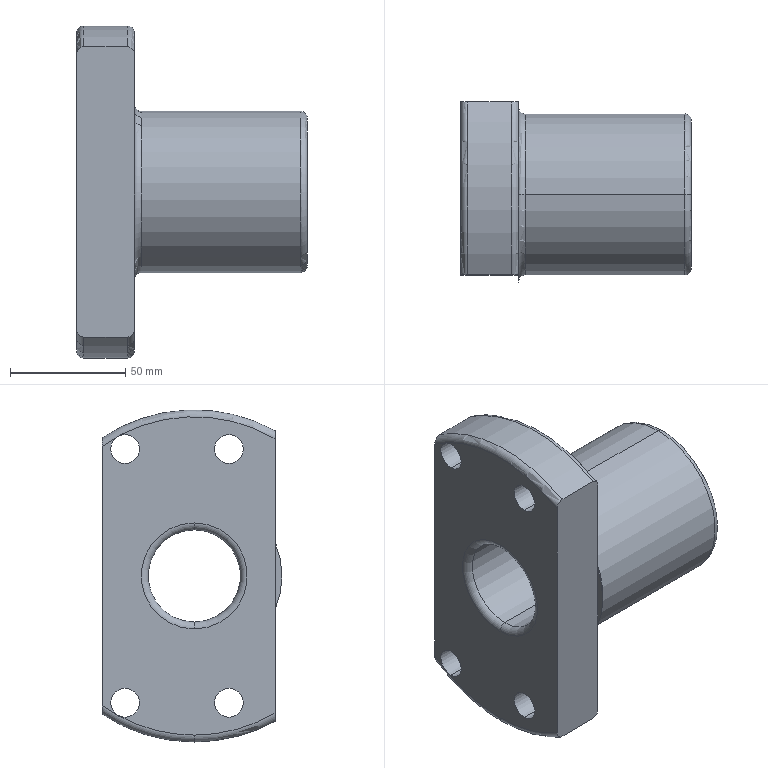Part | SolidWorks | features BaseBody 1 | 1 solid | 35 faces | box 100 x 78 x 144 mm | volume 406652 mm3 | cylinder 15 | torus 14 | plane 6 | commonest cylinder face diameters 12.5 x8 144 x3 40 x2 70 x2
STEP:
#1=CARTESIAN_POINT('',(-75.,30.,-48.75));
#2=VERTEX_POINT('',#1);
#3=CARTESIAN_POINT('',(-75.,30.,-61.25));
#4=VERTEX_POINT('',#3);
#5=CARTESIAN_POINT('',(-75.,30.,-55.));
#6=DIRECTION('',(1.,0.,0.));
#7=DIRECTION('',(0.,0.,-1.));
#8=AXIS2_PLACEMENT_3D('',#5,#6,#7);
#9=CIRCLE('',#8,6.25);
#10=EDGE_CURVE('',#2,#4,#9,.T.);
#11=ORIENTED_EDGE('',*,*,#10,.T.);
#12=CARTESIAN_POINT('',(-100.,30.,-61.25));
#13=VERTEX_POINT('',#12);
#14=CARTESIAN_POINT('',(-70.,30.,-61.25));
#15=DIRECTION('',(-1.,0.,0.));
#16=VECTOR('',#15,1000.);
#17=LINE('',#14,#16);
#18=EDGE_CURVE('',#4,#13,#17,.T.);
#19=ORIENTED_EDGE('',*,*,#18,.T.);
#20=CARTESIAN_POINT('',(-100.,30.,-48.75));
#21=VERTEX_POINT('',#20);
#22=CARTESIAN_POINT('',(-100.,30.,-55.));
#23=DIRECTION('',(-1.,0.,0.));
#24=DIRECTION('',(0.,0.,1.));
#25=AXIS2_PLACEMENT_3D('',#22,#23,#24);
#26=CIRCLE('',#25,6.25);
#27=EDGE_CURVE('',#13,#21,#26,.T.);
#28=ORIENTED_EDGE('',*,*,#27,.T.);
#29=CARTESIAN_POINT('',(-70.,30.,-48.75));
#30=DIRECTION('',(-1.,0.,0.));
#31=VECTOR('',#30,1000.);
#32=LINE('',#29,#31);
#33=EDGE_CURVE('',#2,#21,#32,.T.);
#34=ORIENTED_EDGE('',*,*,#33,.F.);
#35=EDGE_LOOP('',(#11,#19,#28,#34));
#36=FACE_OUTER_BOUND('',#35,.T.);
#37=CARTESIAN_POINT('',(-70.,30.,-55.));
#38=DIRECTION('',(-1.,0.,0.));
#39=DIRECTION('',(0.,0.,1.));
#40=AXIS2_PLACEMENT_3D('',#37,#38,#39);
#41=CYLINDRICAL_SURFACE('',#40,6.25);
#42=ADVANCED_FACE('',(#36),#41,.F.);
#43=CARTESIAN_POINT('',(-75.,30.,61.25));
#44=VERTEX_POINT('',#43);
#45=CARTESIAN_POINT('',(-75.,30.,48.75));
#46=VERTEX_POINT('',#45);
#47=CARTESIAN_POINT('',(-75.,30.,55.));
#48=DIRECTION('',(1.,0.,0.));
#49=DIRECTION('',(0.,0.,-1.));
#50=AXIS2_PLACEMENT_3D('',#47,#48,#49);
#51=CIRCLE('',#50,6.25);
#52=EDGE_CURVE('',#44,#46,#51,.T.);
#53=ORIENTED_EDGE('',*,*,#52,.T.);
#54=CARTESIAN_POINT('',(-100.,30.,48.75));
#55=VERTEX_POINT('',#54);
#56=CARTESIAN_POINT('',(-70.,30.,48.75));
#57=DIRECTION('',(-1.,0.,0.));
#58=VECTOR('',#57,1000.);
#59=LINE('',#56,#58);
#60=EDGE_CURVE('',#46,#55,#59,.T.);
#61=ORIENTED_EDGE('',*,*,#60,.T.);
#62=CARTESIAN_POINT('',(-100.,30.,61.25));
#63=VERTEX_POINT('',#62);
#64=CARTESIAN_POINT('',(-100.,30.,55.));
#65=DIRECTION('',(-1.,0.,0.));
#66=DIRECTION('',(0.,0.,1.));
#67=AXIS2_PLACEMENT_3D('',#64,#65,#66);
#68=CIRCLE('',#67,6.25);
#69=EDGE_CURVE('',#55,#63,#68,.T.);
#70=ORIENTED_EDGE('',*,*,#69,.T.);
#71=CARTESIAN_POINT('',(-70.,30.,61.25));
#72=DIRECTION('',(-1.,0.,0.));
#73=VECTOR('',#72,1000.);
#74=LINE('',#71,#73);
#75=EDGE_CURVE('',#44,#63,#74,.T.);
#76=ORIENTED_EDGE('',*,*,#75,.F.);
#77=EDGE_LOOP('',(#53,#61,#70,#76));
#78=FACE_OUTER_BOUND('',#77,.T.);
#79=CARTESIAN_POINT('',(-70.,30.,55.));
#80=DIRECTION('',(-1.,0.,0.));
#81=DIRECTION('',(0.,0.,1.));
#82=AXIS2_PLACEMENT_3D('',#79,#80,#81);
#83=CYLINDRICAL_SURFACE('',#82,6.25);
#84=ADVANCED_FACE('',(#78),#83,.F.);
#85=CARTESIAN_POINT('',(-75.,-15.,61.25));
#86=VERTEX_POINT('',#85);
#87=CARTESIAN_POINT('',(-75.,-15.,48.75));
#88=VERTEX_POINT('',#87);
#89=CARTESIAN_POINT('',(-75.,-15.,55.));
#90=DIRECTION('',(1.,0.,0.));
#91=DIRECTION('',(0.,0.,-1.));
#92=AXIS2_PLACEMENT_3D('',#89,#90,#91);
#93=CIRCLE('',#92,6.25);
#94=EDGE_CURVE('',#86,#88,#93,.T.);
#95=ORIENTED_EDGE('',*,*,#94,.T.);
#96=CARTESIAN_POINT('',(-100.,-15.,48.75));
#97=VERTEX_POINT('',#96);
#98=CARTESIAN_POINT('',(-70.,-15.,48.75));
#99=DIRECTION('',(-1.,0.,0.));
#100=VECTOR('',#99,1000.);
#101=LINE('',#98,#100);
#102=EDGE_CURVE('',#88,#97,#101,.T.);
#103=ORIENTED_EDGE('',*,*,#102,.T.);
#104=CARTESIAN_POINT('',(-100.,-15.,61.25));
#105=VERTEX_POINT('',#104);
#106=CARTESIAN_POINT('',(-100.,-15.,55.));
#107=DIRECTION('',(-1.,0.,0.));
#108=DIRECTION('',(0.,0.,1.));
#109=AXIS2_PLACEMENT_3D('',#106,#107,#108);
#110=CIRCLE('',#109,6.25);
#111=EDGE_CURVE('',#97,#105,#110,.T.);
#112=ORIENTED_EDGE('',*,*,#111,.T.);
#113=CARTESIAN_POINT('',(-70.,-15.,61.25));
#114=DIRECTION('',(-1.,0.,0.));
#115=VECTOR('',#114,1000.);
#116=LINE('',#113,#115);
#117=EDGE_CURVE('',#86,#105,#116,.T.);
#118=ORIENTED_EDGE('',*,*,#117,.F.);
#119=EDGE_LOOP('',(#95,#103,#112,#118));
#120=FACE_OUTER_BOUND('',#119,.T.);
#121=CARTESIAN_POINT('',(-70.,-15.,55.));
#122=DIRECTION('',(-1.,0.,0.));
#123=DIRECTION('',(0.,0.,1.));
#124=AXIS2_PLACEMENT_3D('',#121,#122,#123);
#125=CYLINDRICAL_SURFACE('',#124,6.25);
#126=ADVANCED_FACE('',(#120),#125,.F.);
#127=CARTESIAN_POINT('',(-75.,-15.,-48.75));
#128=VERTEX_POINT('',#127);
#129=CARTESIAN_POINT('',(-75.,-15.,-61.25));
#130=VERTEX_POINT('',#129);
#131=CARTESIAN_POINT('',(-75.,-15.,-55.));
#132=DIRECTION('',(1.,0.,0.));
#133=DIRECTION('',(0.,0.,-1.));
#134=AXIS2_PLACEMENT_3D('',#131,#132,#133);
#135=CIRCLE('',#134,6.25);
#136=EDGE_CURVE('',#128,#130,#135,.T.);
#137=ORIENTED_EDGE('',*,*,#136,.T.);
#138=CARTESIAN_POINT('',(-100.,-15.,-61.25));
#139=VERTEX_POINT('',#138);
#140=CARTESIAN_POINT('',(-70.,-15.,-61.25));
#141=DIRECTION('',(-1.,0.,0.));
#142=VECTOR('',#141,1000.);
#143=LINE('',#140,#142);
#144=EDGE_CURVE('',#130,#139,#143,.T.);
#145=ORIENTED_EDGE('',*,*,#144,.T.);
#146=CARTESIAN_POINT('',(-100.,-15.,-48.75));
#147=VERTEX_POINT('',#146);
#148=CARTESIAN_POINT('',(-100.,-15.,-55.));
#149=DIRECTION('',(-1.,0.,0.));
#150=DIRECTION('',(0.,0.,1.));
#151=AXIS2_PLACEMENT_3D('',#148,#149,#150);
#152=CIRCLE('',#151,6.25);
#153=EDGE_CURVE('',#139,#147,#152,.T.);
#154=ORIENTED_EDGE('',*,*,#153,.T.);
#155=CARTESIAN_POINT('',(-70.,-15.,-48.75));
#156=DIRECTION('',(-1.,0.,0.));
#157=VECTOR('',#156,1000.);
#158=LINE('',#155,#157);
#159=EDGE_CURVE('',#128,#147,#158,.T.);
#160=ORIENTED_EDGE('',*,*,#159,.F.);
#161=EDGE_LOOP('',(#137,#145,#154,#160));
#162=FACE_OUTER_BOUND('',#161,.T.);
#163=CARTESIAN_POINT('',(-70.,-15.,-55.));
#164=DIRECTION('',(-1.,0.,0.));
#165=DIRECTION('',(0.,0.,1.));
#166=AXIS2_PLACEMENT_3D('',#163,#164,#165);
#167=CYLINDRICAL_SURFACE('',#166,6.25);
#168=ADVANCED_FACE('',(#162),#167,.F.);
#169=CARTESIAN_POINT('',(-3.,0.,-35.));
#170=VERTEX_POINT('',#169);
#171=CARTESIAN_POINT('',(-3.,0.,35.));
#172=VERTEX_POINT('',#171);
#173=CARTESIAN_POINT('',(-3.,0.,0.));
#174=DIRECTION('',(1.,0.,0.));
#175=DIRECTION('',(0.,0.,-1.));
#176=AXIS2_PLACEMENT_3D('',#173,#174,#175);
#177=CIRCLE('',#176,35.);
#178=EDGE_CURVE('',#170,#172,#177,.T.);
#179=ORIENTED_EDGE('',*,*,#178,.T.);
#180=CARTESIAN_POINT('',(0.,0.,32.));
#181=VERTEX_POINT('',#180);
#182=CARTESIAN_POINT('',(-3.,0.,32.));
#183=DIRECTION('',(0.,1.,0.));
#184=DIRECTION('',(0.,0.,1.));
#185=AXIS2_PLACEMENT_3D('',#182,#183,#184);
#186=CIRCLE('',#185,3.);
#187=EDGE_CURVE('',#172,#181,#186,.T.);
#188=ORIENTED_EDGE('',*,*,#187,.T.);
#189=CARTESIAN_POINT('',(0.,0.,-32.));
#190=VERTEX_POINT('',#189);
#191=CARTESIAN_POINT('',(0.,0.,0.));
#192=DIRECTION('',(1.,0.,0.));
#193=DIRECTION('',(0.,0.,-1.));
#194=AXIS2_PLACEMENT_3D('',#191,#192,#193);
#195=CIRCLE('',#194,32.);
#196=EDGE_CURVE('',#190,#181,#195,.T.);
#197=ORIENTED_EDGE('',*,*,#196,.F.);
#198=CARTESIAN_POINT('',(-3.,0.,-32.));
#199=DIRECTION('',(0.,-1.,0.));
#200=DIRECTION('',(0.,0.,-1.));
#201=AXIS2_PLACEMENT_3D('',#198,#199,#200);
#202=CIRCLE('',#201,3.);
#203=EDGE_CURVE('',#170,#190,#202,.T.);
#204=ORIENTED_EDGE('',*,*,#203,.F.);
#205=EDGE_LOOP('',(#179,#188,#197,#204));
#206=FACE_OUTER_BOUND('',#205,.T.);
#207=CARTESIAN_POINT('',(-3.,0.,0.));
#208=DIRECTION('',(1.,0.,0.));
#209=DIRECTION('',(0.,0.,-1.));
#210=AXIS2_PLACEMENT_3D('',#207,#208,#209);
#211=TOROIDAL_SURFACE('',#210,32.,3.);
#212=ADVANCED_FACE('',(#206),#211,.T.);
#213=CARTESIAN_POINT('',(-72.,0.,-35.));
#214=VERTEX_POINT('',#213);
#215=CARTESIAN_POINT('',(-72.,0.,35.));
#216=VERTEX_POINT('',#215);
#217=CARTESIAN_POINT('',(-72.,0.,0.));
#218=DIRECTION('',(1.,0.,0.));
#219=DIRECTION('',(0.,0.,-1.));
#220=AXIS2_PLACEMENT_3D('',#217,#218,#219);
#221=CIRCLE('',#220,35.);
#222=EDGE_CURVE('',#214,#216,#221,.T.);
#223=ORIENTED_EDGE('',*,*,#222,.T.);
#224=CARTESIAN_POINT('',(0.,0.,35.));
#225=DIRECTION('',(1.,0.,0.));
#226=VECTOR('',#225,1000.);
#227=LINE('',#224,#226);
#228=EDGE_CURVE('',#216,#172,#227,.T.);
#229=ORIENTED_EDGE('',*,*,#228,.T.);
#230=ORIENTED_EDGE('',*,*,#178,.F.);
#231=CARTESIAN_POINT('',(0.,0.,-35.));
#232=DIRECTION('',(1.,0.,0.));
#233=VECTOR('',#232,1000.);
#234=LINE('',#231,#233);
#235=EDGE_CURVE('',#214,#170,#234,.T.);
#236=ORIENTED_EDGE('',*,*,#235,.F.);
#237=EDGE_LOOP('',(#223,#229,#230,#236));
#238=FACE_OUTER_BOUND('',#237,.T.);
#239=CARTESIAN_POINT('',(0.,0.,0.));
#240=DIRECTION('',(1.,0.,0.));
#241=DIRECTION('',(0.,0.,-1.));
#242=AXIS2_PLACEMENT_3D('',#239,#240,#241);
#243=CYLINDRICAL_SURFACE('',#242,35.);
#244=ADVANCED_FACE('',(#238),#243,.T.);
#245=CARTESIAN_POINT('',(-72.,0.,0.));
#246=DIRECTION('',(1.,0.,0.));
#247=DIRECTION('',(0.,0.,-1.));
#248=AXIS2_PLACEMENT_3D('',#245,#246,#247);
#249=CIRCLE('',#248,35.);
#250=EDGE_CURVE('',#216,#214,#249,.T.);
#251=ORIENTED_EDGE('',*,*,#250,.F.);
#252=CARTESIAN_POINT('',(-75.,0.,38.));
#253=VERTEX_POINT('',#252);
#254=CARTESIAN_POINT('',(-72.,0.,38.));
#255=DIRECTION('',(0.,1.,0.));
#256=DIRECTION('',(0.,0.,1.));
#257=AXIS2_PLACEMENT_3D('',#254,#255,#256);
#258=CIRCLE('',#257,3.);
#259=EDGE_CURVE('',#216,#253,#258,.T.);
#260=ORIENTED_EDGE('',*,*,#259,.T.);
#261=CARTESIAN_POINT('',(-75.,-35.,14.799));
#262=VERTEX_POINT('',#261);
#263=CARTESIAN_POINT('',(-75.,0.,0.));
#264=DIRECTION('',(1.,0.,0.));
#265=DIRECTION('',(0.,0.,-1.));
#266=AXIS2_PLACEMENT_3D('',#263,#264,#265);
#267=CIRCLE('',#266,38.);
#268=EDGE_CURVE('',#253,#262,#267,.T.);
#269=ORIENTED_EDGE('',*,*,#268,.T.);
#270=CARTESIAN_POINT('',(-75.,-35.,-14.799));
#271=VERTEX_POINT('',#270);
#272=CARTESIAN_POINT('',(-75.,0.,0.));
#273=DIRECTION('',(1.,0.,0.));
#274=DIRECTION('',(0.,0.,-1.));
#275=AXIS2_PLACEMENT_3D('',#272,#273,#274);
#276=CIRCLE('',#275,38.);
#277=EDGE_CURVE('',#262,#271,#276,.T.);
#278=ORIENTED_EDGE('',*,*,#277,.T.);
#279=CARTESIAN_POINT('',(-75.,0.,-38.));
#280=VERTEX_POINT('',#279);
#281=CARTESIAN_POINT('',(-75.,0.,0.));
#282=DIRECTION('',(1.,0.,0.));
#283=DIRECTION('',(0.,0.,-1.));
#284=AXIS2_PLACEMENT_3D('',#281,#282,#283);
#285=CIRCLE('',#284,38.);
#286=EDGE_CURVE('',#271,#280,#285,.T.);
#287=ORIENTED_EDGE('',*,*,#286,.T.);
#288=CARTESIAN_POINT('',(-72.,0.,-38.));
#289=DIRECTION('',(0.,-1.,0.));
#290=DIRECTION('',(0.,0.,-1.));
#291=AXIS2_PLACEMENT_3D('',#288,#289,#290);
#292=CIRCLE('',#291,3.);
#293=EDGE_CURVE('',#214,#280,#292,.T.);
#294=ORIENTED_EDGE('',*,*,#293,.F.);
#295=EDGE_LOOP('',(#251,#260,#269,#278,#287,#294));
#296=FACE_OUTER_BOUND('',#295,.T.);
#297=CARTESIAN_POINT('',(-72.,0.,0.));
#298=DIRECTION('',(1.,0.,0.));
#299=DIRECTION('',(0.,0.,-1.));
#300=AXIS2_PLACEMENT_3D('',#297,#298,#299);
#301=TOROIDAL_SURFACE('',#300,38.,3.);
#302=ADVANCED_FACE('',(#296),#301,.F.);
#303=CARTESIAN_POINT('',(-97.,0.,-20.));
#304=VERTEX_POINT('',#303);
#305=CARTESIAN_POINT('',(-97.,0.,20.));
#306=VERTEX_POINT('',#305);
#307=CARTESIAN_POINT('',(-97.,0.,0.));
#308=DIRECTION('',(1.,0.,0.));
#309=DIRECTION('',(0.,0.,-1.));
#310=AXIS2_PLACEMENT_3D('',#307,#308,#309);
#311=CIRCLE('',#310,20.);
#312=EDGE_CURVE('',#304,#306,#311,.T.);
#313=ORIENTED_EDGE('',*,*,#312,.T.);
#314=CARTESIAN_POINT('',(-100.,0.,23.));
#315=VERTEX_POINT('',#314);
#316=CARTESIAN_POINT('',(-97.,0.,23.));
#317=DIRECTION('',(0.,1.,0.));
#318=DIRECTION('',(0.,0.,1.));
#319=AXIS2_PLACEMENT_3D('',#316,#317,#318);
#320=CIRCLE('',#319,3.);
#321=EDGE_CURVE('',#306,#315,#320,.T.);
#322=ORIENTED_EDGE('',*,*,#321,.T.);
#323=CARTESIAN_POINT('',(-100.,0.,-23.));
#324=VERTEX_POINT('',#323);
#325=CARTESIAN_POINT('',(-100.,0.,0.));
#326=DIRECTION('',(1.,0.,0.));
#327=DIRECTION('',(0.,0.,-1.));
#328=AXIS2_PLACEMENT_3D('',#325,#326,#327);
#329=CIRCLE('',#328,23.);
#330=EDGE_CURVE('',#324,#315,#329,.T.);
#331=ORIENTED_EDGE('',*,*,#330,.F.);
#332=CARTESIAN_POINT('',(-97.,0.,-23.));
#333=DIRECTION('',(0.,-1.,0.));
#334=DIRECTION('',(0.,0.,-1.));
#335=AXIS2_PLACEMENT_3D('',#332,#333,#334);
#336=CIRCLE('',#335,3.);
#337=EDGE_CURVE('',#304,#324,#336,.T.);
#338=ORIENTED_EDGE('',*,*,#337,.F.);
#339=EDGE_LOOP('',(#313,#322,#331,#338));
#340=FACE_OUTER_BOUND('',#339,.T.);
#341=CARTESIAN_POINT('',(-97.,0.,0.));
#342=DIRECTION('',(1.,0.,0.));
#343=DIRECTION('',(0.,0.,-1.));
#344=AXIS2_PLACEMENT_3D('',#341,#342,#343);
#345=TOROIDAL_SURFACE('',#344,23.,3.);
#346=ADVANCED_FACE('',(#340),#345,.T.);
#347=CARTESIAN_POINT('',(-97.,0.,0.));
#348=DIRECTION('',(1.,0.,0.));
#349=DIRECTION('',(0.,0.,-1.));
#350=AXIS2_PLACEMENT_3D('',#347,#348,#349);
#351=CIRCLE('',#350,20.);
#352=EDGE_CURVE('',#306,#304,#351,.T.);
#353=ORIENTED_EDGE('',*,*,#352,.F.);
#354=CARTESIAN_POINT('',(-3.,0.,20.));
#355=VERTEX_POINT('',#354);
#356=CARTESIAN_POINT('',(0.,0.,20.));
#357=DIRECTION('',(1.,0.,0.));
#358=VECTOR('',#357,1000.);
#359=LINE('',#356,#358);
#360=EDGE_CURVE('',#306,#355,#359,.T.);
#361=ORIENTED_EDGE('',*,*,#360,.T.);
#362=CARTESIAN_POINT('',(-3.,0.,-20.));
#363=VERTEX_POINT('',#362);
#364=CARTESIAN_POINT('',(-3.,0.,0.));
#365=DIRECTION('',(1.,0.,0.));
#366=DIRECTION('',(0.,0.,-1.));
#367=AXIS2_PLACEMENT_3D('',#364,#365,#366);
#368=CIRCLE('',#367,20.);
#369=EDGE_CURVE('',#355,#363,#368,.T.);
#370=ORIENTED_EDGE('',*,*,#369,.T.);
#371=CARTESIAN_POINT('',(0.,0.,-20.));
#372=DIRECTION('',(1.,0.,0.));
#373=VECTOR('',#372,1000.);
#374=LINE('',#371,#373);
#375=EDGE_CURVE('',#304,#363,#374,.T.);
#376=ORIENTED_EDGE('',*,*,#375,.F.);
#377=EDGE_LOOP('',(#353,#361,#370,#376));
#378=FACE_OUTER_BOUND('',#377,.T.);
#379=CARTESIAN_POINT('',(0.,0.,0.));
#380=DIRECTION('',(1.,0.,0.));
#381=DIRECTION('',(0.,0.,-1.));
#382=AXIS2_PLACEMENT_3D('',#379,#380,#381);
#383=CYLINDRICAL_SURFACE('',#382,20.);
#384=ADVANCED_FACE('',(#378),#383,.F.);
#385=CARTESIAN_POINT('',(0.,0.,-23.));
#386=VERTEX_POINT('',#385);
#387=CARTESIAN_POINT('',(0.,0.,23.));
#388=VERTEX_POINT('',#387);
#389=CARTESIAN_POINT('',(0.,0.,0.));
#390=DIRECTION('',(1.,0.,0.));
#391=DIRECTION('',(0.,0.,-1.));
#392=AXIS2_PLACEMENT_3D('',#389,#390,#391);
#393=CIRCLE('',#392,23.);
#394=EDGE_CURVE('',#386,#388,#393,.T.);
#395=ORIENTED_EDGE('',*,*,#394,.T.);
#396=CARTESIAN_POINT('',(-3.,0.,23.));
#397=DIRECTION('',(0.,1.,0.));
#398=DIRECTION('',(0.,0.,1.));
#399=AXIS2_PLACEMENT_3D('',#396,#397,#398);
#400=CIRCLE('',#399,3.);
#401=EDGE_CURVE('',#388,#355,#400,.T.);
#402=ORIENTED_EDGE('',*,*,#401,.T.);
#403=CARTESIAN_POINT('',(-3.,0.,0.));
#404=DIRECTION('',(1.,0.,0.));
#405=DIRECTION('',(0.,0.,-1.));
#406=AXIS2_PLACEMENT_3D('',#403,#404,#405);
#407=CIRCLE('',#406,20.);
#408=EDGE_CURVE('',#363,#355,#407,.T.);
#409=ORIENTED_EDGE('',*,*,#408,.F.);
#410=CARTESIAN_POINT('',(-3.,0.,-23.));
#411=DIRECTION('',(0.,-1.,0.));
#412=DIRECTION('',(0.,0.,-1.));
#413=AXIS2_PLACEMENT_3D('',#410,#411,#412);
#414=CIRCLE('',#413,3.);
#415=EDGE_CURVE('',#386,#363,#414,.T.);
#416=ORIENTED_EDGE('',*,*,#415,.F.);
#417=EDGE_LOOP('',(#395,#402,#409,#416));
#418=FACE_OUTER_BOUND('',#417,.T.);
#419=CARTESIAN_POINT('',(-3.,0.,0.));
#420=DIRECTION('',(1.,0.,0.));
#421=DIRECTION('',(0.,0.,-1.));
#422=AXIS2_PLACEMENT_3D('',#419,#420,#421);
#423=TOROIDAL_SURFACE('',#422,23.,3.);
#424=ADVANCED_FACE('',(#418),#423,.T.);
#425=CARTESIAN_POINT('',(-78.,-35.,-62.921));
#426=VERTEX_POINT('',#425);
#427=CARTESIAN_POINT('',(-78.,0.,-72.));
#428=VERTEX_POINT('',#427);
#429=CARTESIAN_POINT('',(-78.,0.,0.));
#430=DIRECTION('',(1.,0.,0.));
#431=DIRECTION('',(0.,0.,-1.));
#432=AXIS2_PLACEMENT_3D('',#429,#430,#431);
#433=CIRCLE('',#432,72.);
#434=EDGE_CURVE('',#426,#428,#433,.T.);
#435=ORIENTED_EDGE('',*,*,#434,.T.);
#436=CARTESIAN_POINT('',(-75.,0.,-69.));
#437=VERTEX_POINT('',#436);
#438=CARTESIAN_POINT('',(-78.,0.,-69.));
#439=DIRECTION('',(0.,-1.,0.));
#440=DIRECTION('',(0.,0.,-1.));
#441=AXIS2_PLACEMENT_3D('',#438,#439,#440);
#442=CIRCLE('',#441,3.);
#443=EDGE_CURVE('',#428,#437,#442,.T.);
#444=ORIENTED_EDGE('',*,*,#443,.T.);
#445=CARTESIAN_POINT('',(-75.,-35.,-59.464));
#446=VERTEX_POINT('',#445);
#447=CARTESIAN_POINT('',(-75.,0.,0.));
#448=DIRECTION('',(1.,0.,0.));
#449=DIRECTION('',(0.,0.,-1.));
#450=AXIS2_PLACEMENT_3D('',#447,#448,#449);
#451=CIRCLE('',#450,69.);
#452=EDGE_CURVE('',#446,#437,#451,.T.);
#453=ORIENTED_EDGE('',*,*,#452,.F.);
#454=CARTESIAN_POINT('',(-78.,-35.,-62.921));
#455=CARTESIAN_POINT('',(-77.789,-35.,-62.921));
#456=CARTESIAN_POINT('',(-77.576,-35.,-62.895));
#457=CARTESIAN_POINT('',(-77.163,-35.,-62.793));
#458=CARTESIAN_POINT('',(-76.965,-35.,-62.718));
#459=CARTESIAN_POINT('',(-76.586,-35.,-62.525));
#460=CARTESIAN_POINT('',(-76.407,-35.,-62.406));
#461=CARTESIAN_POINT('',(-76.078,-35.,-62.132));
#462=CARTESIAN_POINT('',(-75.931,-35.,-61.982));
#463=CARTESIAN_POINT('',(-75.667,-35.,-61.655));
#464=CARTESIAN_POINT('',(-75.55,-35.,-61.477));
#465=CARTESIAN_POINT('',(-75.349,-35.,-61.103));
#466=CARTESIAN_POINT('',(-75.266,-35.,-60.91));
#467=CARTESIAN_POINT('',(-75.133,-35.,-60.51));
#468=CARTESIAN_POINT('',(-75.083,-35.,-60.302));
#469=CARTESIAN_POINT('',(-75.016,-35.,-59.885));
#470=CARTESIAN_POINT('',(-75.,-35.,-59.675));
#471=CARTESIAN_POINT('',(-75.,-35.,-59.464));
#472=B_SPLINE_CURVE_WITH_KNOTS('',3,(#454,#455,#456,#457,#458,#459,#460,#461,#462,#463,#464,#465,#466,#467,#468,#469,#470,#471),.UNSPECIFIED.,.F.,.F.,(4,2,2,2,2,2,2,2,4),(0.01836,0.01899,0.01962,0.02025,0.02088,0.02151,0.02214,0.02277,0.0234),.UNSPECIFIED.);
#473=EDGE_CURVE('',#426,#446,#472,.T.);
#474=ORIENTED_EDGE('',*,*,#473,.F.);
#475=EDGE_LOOP('',(#435,#444,#453,#474));
#476=FACE_OUTER_BOUND('',#475,.T.);
#477=CARTESIAN_POINT('',(-78.,0.,0.));
#478=DIRECTION('',(1.,0.,0.));
#479=DIRECTION('',(0.,0.,-1.));
#480=AXIS2_PLACEMENT_3D('',#477,#478,#479);
#481=TOROIDAL_SURFACE('',#480,69.,3.);
#482=ADVANCED_FACE('',(#476),#481,.T.);
#483=CARTESIAN_POINT('',(-97.,-35.,-62.921));
#484=VERTEX_POINT('',#483);
#485=CARTESIAN_POINT('',(-97.,0.,-72.));
#486=VERTEX_POINT('',#485);
#487=CARTESIAN_POINT('',(-97.,0.,0.));
#488=DIRECTION('',(1.,0.,0.));
#489=DIRECTION('',(0.,0.,-1.));
#490=AXIS2_PLACEMENT_3D('',#487,#488,#489);
#491=CIRCLE('',#490,72.);
#492=EDGE_CURVE('',#484,#486,#491,.T.);
#493=ORIENTED_EDGE('',*,*,#492,.T.);
#494=CARTESIAN_POINT('',(0.,0.,-72.));
#495=DIRECTION('',(1.,0.,0.));
#496=VECTOR('',#495,1000.);
#497=LINE('',#494,#496);
#498=EDGE_CURVE('',#486,#428,#497,.T.);
#499=ORIENTED_EDGE('',*,*,#498,.T.);
#500=ORIENTED_EDGE('',*,*,#434,.F.);
#501=CARTESIAN_POINT('',(56.168,-35.,-62.921));
#502=DIRECTION('',(-1.,0.,0.));
#503=VECTOR('',#502,1000.);
#504=LINE('',#501,#503);
#505=EDGE_CURVE('',#426,#484,#504,.T.);
#506=ORIENTED_EDGE('',*,*,#505,.T.);
#507=EDGE_LOOP('',(#493,#499,#500,#506));
#508=FACE_OUTER_BOUND('',#507,.T.);
#509=CARTESIAN_POINT('',(0.,0.,0.));
#510=DIRECTION('',(1.,0.,0.));
#511=DIRECTION('',(0.,0.,-1.));
#512=AXIS2_PLACEMENT_3D('',#509,#510,#511);
#513=CYLINDRICAL_SURFACE('',#512,72.);
#514=ADVANCED_FACE('',(#508),#513,.T.);
#515=CARTESIAN_POINT('',(-100.,-35.,-59.464));
#516=VERTEX_POINT('',#515);
#517=CARTESIAN_POINT('',(-100.,0.,-69.));
#518=VERTEX_POINT('',#517);
#519=CARTESIAN_POINT('',(-100.,0.,0.));
#520=DIRECTION('',(1.,0.,0.));
#521=DIRECTION('',(0.,0.,-1.));
#522=AXIS2_PLACEMENT_3D('',#519,#520,#521);
#523=CIRCLE('',#522,69.);
#524=EDGE_CURVE('',#516,#518,#523,.T.);
#525=ORIENTED_EDGE('',*,*,#524,.T.);
#526=CARTESIAN_POINT('',(-97.,0.,-69.));
#527=DIRECTION('',(0.,-1.,0.));
#528=DIRECTION('',(0.,0.,-1.));
#529=AXIS2_PLACEMENT_3D('',#526,#527,#528);
#530=CIRCLE('',#529,3.);
#531=EDGE_CURVE('',#518,#486,#530,.T.);
#532=ORIENTED_EDGE('',*,*,#531,.T.);
#533=ORIENTED_EDGE('',*,*,#492,.F.);
#534=CARTESIAN_POINT('',(-100.,-35.,-59.464));
#535=CARTESIAN_POINT('',(-100.,-35.,-59.886));
#536=CARTESIAN_POINT('',(-99.933,-35.,-60.313));
#537=CARTESIAN_POINT('',(-99.733,-35.,-60.912));
#538=CARTESIAN_POINT('',(-99.65,-35.,-61.106));
#539=CARTESIAN_POINT('',(-99.447,-35.,-61.481));
#540=CARTESIAN_POINT('',(-99.33,-35.,-61.658));
#541=CARTESIAN_POINT('',(-99.065,-35.,-61.986));
#542=CARTESIAN_POINT('',(-98.917,-35.,-62.137));
#543=CARTESIAN_POINT('',(-98.588,-35.,-62.409));
#544=CARTESIAN_POINT('',(-98.412,-35.,-62.526));
#545=CARTESIAN_POINT('',(-98.035,-35.,-62.718));
#546=CARTESIAN_POINT('',(-97.833,-35.,-62.794));
#547=CARTESIAN_POINT('',(-97.424,-35.,-62.895));
#548=CARTESIAN_POINT('',(-97.214,-35.,-62.921));
#549=CARTESIAN_POINT('',(-97.,-35.,-62.921));
#550=B_SPLINE_CURVE_WITH_KNOTS('',3,(#534,#535,#536,#537,#538,#539,#540,#541,#542,#543,#544,#545,#546,#547,#548,#549),.UNSPECIFIED.,.F.,.F.,(4,2,2,2,2,2,2,4),(0.01716,0.01842,0.01906,0.01969,0.02032,0.02096,0.02159,0.02222),.UNSPECIFIED.);
#551=EDGE_CURVE('',#516,#484,#550,.T.);
#552=ORIENTED_EDGE('',*,*,#551,.F.);
#553=EDGE_LOOP('',(#525,#532,#533,#552));
#554=FACE_OUTER_BOUND('',#553,.T.);
#555=CARTESIAN_POINT('',(-97.,0.,0.));
#556=DIRECTION('',(1.,0.,0.));
#557=DIRECTION('',(0.,0.,-1.));
#558=AXIS2_PLACEMENT_3D('',#555,#556,#557);
#559=TOROIDAL_SURFACE('',#558,69.,3.);
#560=ADVANCED_FACE('',(#554),#559,.T.);
#561=ORIENTED_EDGE('',*,*,#531,.F.);
#562=CARTESIAN_POINT('',(-100.,40.,-56.223));
#563=VERTEX_POINT('',#562);
#564=CARTESIAN_POINT('',(-100.,0.,0.));
#565=DIRECTION('',(1.,0.,0.));
#566=DIRECTION('',(0.,0.,-1.));
#567=AXIS2_PLACEMENT_3D('',#564,#565,#566);
#568=CIRCLE('',#567,69.);
#569=EDGE_CURVE('',#518,#563,#568,.T.);
#570=ORIENTED_EDGE('',*,*,#569,.T.);
#571=CARTESIAN_POINT('',(-97.,40.,-59.867));
#572=VERTEX_POINT('',#571);
#573=CARTESIAN_POINT('',(-97.,40.,-59.867));
#574=CARTESIAN_POINT('',(-97.218,40.,-59.867));
#575=CARTESIAN_POINT('',(-97.439,40.,-59.837));
#576=CARTESIAN_POINT('',(-97.86,40.,-59.725));
#577=CARTESIAN_POINT('',(-98.067,40.,-59.64));
#578=CARTESIAN_POINT('',(-98.449,40.,-59.428));
#579=CARTESIAN_POINT('',(-98.628,40.,-59.298));
#580=CARTESIAN_POINT('',(-98.953,40.,-59.006));
#581=CARTESIAN_POINT('',(-99.098,40.,-58.845));
#582=CARTESIAN_POINT('',(-99.357,40.,-58.498));
#583=CARTESIAN_POINT('',(-99.472,40.,-58.309));
#584=CARTESIAN_POINT('',(-99.666,40.,-57.919));
#585=CARTESIAN_POINT('',(-99.746,40.,-57.717));
#586=CARTESIAN_POINT('',(-99.873,40.,-57.301));
#587=CARTESIAN_POINT('',(-99.921,40.,-57.086));
#588=CARTESIAN_POINT('',(-99.984,40.,-56.656));
#589=CARTESIAN_POINT('',(-100.,40.,-56.44));
#590=CARTESIAN_POINT('',(-100.,40.,-56.223));
#591=B_SPLINE_CURVE_WITH_KNOTS('',3,(#573,#574,#575,#576,#577,#578,#579,#580,#581,#582,#583,#584,#585,#586,#587,#588,#589,#590),.UNSPECIFIED.,.F.,.F.,(4,2,2,2,2,2,2,2,4),(0.01904,0.01969,0.02034,0.02099,0.02164,0.02229,0.02294,0.02358,0.02423),.UNSPECIFIED.);
#592=EDGE_CURVE('',#572,#563,#591,.T.);
#593=ORIENTED_EDGE('',*,*,#592,.F.);
#594=CARTESIAN_POINT('',(-97.,0.,0.));
#595=DIRECTION('',(1.,0.,0.));
#596=DIRECTION('',(0.,0.,-1.));
#597=AXIS2_PLACEMENT_3D('',#594,#595,#596);
#598=CIRCLE('',#597,72.);
#599=EDGE_CURVE('',#486,#572,#598,.T.);
#600=ORIENTED_EDGE('',*,*,#599,.F.);
#601=EDGE_LOOP('',(#561,#570,#593,#600));
#602=FACE_OUTER_BOUND('',#601,.T.);
#603=CARTESIAN_POINT('',(-97.,0.,0.));
#604=DIRECTION('',(1.,0.,0.));
#605=DIRECTION('',(0.,0.,-1.));
#606=AXIS2_PLACEMENT_3D('',#603,#604,#605);
#607=TOROIDAL_SURFACE('',#606,69.,3.);
#608=ADVANCED_FACE('',(#602),#607,.T.);
#609=ORIENTED_EDGE('',*,*,#498,.F.);
#610=ORIENTED_EDGE('',*,*,#599,.T.);
#611=CARTESIAN_POINT('',(-78.,40.,-59.867));
#612=VERTEX_POINT('',#611);
#613=CARTESIAN_POINT('',(56.168,40.,-59.867));
#614=DIRECTION('',(-1.,0.,0.));
#615=VECTOR('',#614,1000.);
#616=LINE('',#613,#615);
#617=EDGE_CURVE('',#612,#572,#616,.T.);
#618=ORIENTED_EDGE('',*,*,#617,.F.);
#619=CARTESIAN_POINT('',(-78.,0.,0.));
#620=DIRECTION('',(1.,0.,0.));
#621=DIRECTION('',(0.,0.,-1.));
#622=AXIS2_PLACEMENT_3D('',#619,#620,#621);
#623=CIRCLE('',#622,72.);
#624=EDGE_CURVE('',#428,#612,#623,.T.);
#625=ORIENTED_EDGE('',*,*,#624,.F.);
#626=EDGE_LOOP('',(#609,#610,#618,#625));
#627=FACE_OUTER_BOUND('',#626,.T.);
#628=CARTESIAN_POINT('',(0.,0.,0.));
#629=DIRECTION('',(1.,0.,0.));
#630=DIRECTION('',(0.,0.,-1.));
#631=AXIS2_PLACEMENT_3D('',#628,#629,#630);
#632=CYLINDRICAL_SURFACE('',#631,72.);
#633=ADVANCED_FACE('',(#627),#632,.T.);
#634=ORIENTED_EDGE('',*,*,#443,.F.);
#635=ORIENTED_EDGE('',*,*,#624,.T.);
#636=CARTESIAN_POINT('',(-75.,40.,-56.223));
#637=VERTEX_POINT('',#636);
#638=CARTESIAN_POINT('',(-75.,40.,-56.223));
#639=CARTESIAN_POINT('',(-75.,40.,-56.662));
#640=CARTESIAN_POINT('',(-75.062,40.,-57.091));
#641=CARTESIAN_POINT('',(-75.254,40.,-57.717));
#642=CARTESIAN_POINT('',(-75.336,40.,-57.922));
#643=CARTESIAN_POINT('',(-75.529,40.,-58.311));
#644=CARTESIAN_POINT('',(-75.642,40.,-58.497));
#645=CARTESIAN_POINT('',(-75.904,40.,-58.848));
#646=CARTESIAN_POINT('',(-76.052,40.,-59.012));
#647=CARTESIAN_POINT('',(-76.381,40.,-59.305));
#648=CARTESIAN_POINT('',(-76.558,40.,-59.432));
#649=CARTESIAN_POINT('',(-76.939,40.,-59.642));
#650=CARTESIAN_POINT('',(-77.145,40.,-59.726));
#651=CARTESIAN_POINT('',(-77.564,40.,-59.838));
#652=CARTESIAN_POINT('',(-77.78,40.,-59.867));
#653=CARTESIAN_POINT('',(-78.,40.,-59.867));
#654=B_SPLINE_CURVE_WITH_KNOTS('',3,(#638,#639,#640,#641,#642,#643,#644,#645,#646,#647,#648,#649,#650,#651,#652,#653),.UNSPECIFIED.,.F.,.F.,(4,2,2,2,2,2,2,4),(0.01763,0.01893,0.01958,0.02023,0.02088,0.02154,0.02219,0.02284),.UNSPECIFIED.);
#655=EDGE_CURVE('',#637,#612,#654,.T.);
#656=ORIENTED_EDGE('',*,*,#655,.F.);
#657=CARTESIAN_POINT('',(-75.,0.,0.));
#658=DIRECTION('',(1.,0.,0.));
#659=DIRECTION('',(0.,0.,-1.));
#660=AXIS2_PLACEMENT_3D('',#657,#658,#659);
#661=CIRCLE('',#660,69.);
#662=EDGE_CURVE('',#437,#637,#661,.T.);
#663=ORIENTED_EDGE('',*,*,#662,.F.);
#664=EDGE_LOOP('',(#634,#635,#656,#663));
#665=FACE_OUTER_BOUND('',#664,.T.);
#666=CARTESIAN_POINT('',(-78.,0.,0.));
#667=DIRECTION('',(1.,0.,0.));
#668=DIRECTION('',(0.,0.,-1.));
#669=AXIS2_PLACEMENT_3D('',#666,#667,#668);
#670=TOROIDAL_SURFACE('',#669,69.,3.);
#671=ADVANCED_FACE('',(#665),#670,.T.);
#672=ORIENTED_EDGE('',*,*,#401,.F.);
#673=CARTESIAN_POINT('',(0.,0.,0.));
#674=DIRECTION('',(1.,0.,0.));
#675=DIRECTION('',(0.,0.,-1.));
#676=AXIS2_PLACEMENT_3D('',#673,#674,#675);
#677=CIRCLE('',#676,23.);
#678=EDGE_CURVE('',#388,#386,#677,.T.);
#679=ORIENTED_EDGE('',*,*,#678,.T.);
#680=ORIENTED_EDGE('',*,*,#415,.T.);
#681=ORIENTED_EDGE('',*,*,#369,.F.);
#682=EDGE_LOOP('',(#672,#679,#680,#681));
#683=FACE_OUTER_BOUND('',#682,.T.);
#684=CARTESIAN_POINT('',(-3.,0.,0.));
#685=DIRECTION('',(1.,0.,0.));
#686=DIRECTION('',(0.,0.,-1.));
#687=AXIS2_PLACEMENT_3D('',#684,#685,#686);
#688=TOROIDAL_SURFACE('',#687,23.,3.);
#689=ADVANCED_FACE('',(#683),#688,.T.);
#690=ORIENTED_EDGE('',*,*,#360,.F.);
#691=ORIENTED_EDGE('',*,*,#312,.F.);
#692=ORIENTED_EDGE('',*,*,#375,.T.);
#693=ORIENTED_EDGE('',*,*,#408,.T.);
#694=EDGE_LOOP('',(#690,#691,#692,#693));
#695=FACE_OUTER_BOUND('',#694,.T.);
#696=CARTESIAN_POINT('',(0.,0.,0.));
#697=DIRECTION('',(1.,0.,0.));
#698=DIRECTION('',(0.,0.,-1.));
#699=AXIS2_PLACEMENT_3D('',#696,#697,#698);
#700=CYLINDRICAL_SURFACE('',#699,20.);
#701=ADVANCED_FACE('',(#695),#700,.F.);
#702=ORIENTED_EDGE('',*,*,#321,.F.);
#703=ORIENTED_EDGE('',*,*,#352,.T.);
#704=ORIENTED_EDGE('',*,*,#337,.T.);
#705=CARTESIAN_POINT('',(-100.,0.,0.));
#706=DIRECTION('',(1.,0.,0.));
#707=DIRECTION('',(0.,0.,-1.));
#708=AXIS2_PLACEMENT_3D('',#705,#706,#707);
#709=CIRCLE('',#708,23.);
#710=EDGE_CURVE('',#315,#324,#709,.T.);
#711=ORIENTED_EDGE('',*,*,#710,.F.);
#712=EDGE_LOOP('',(#702,#703,#704,#711));
#713=FACE_OUTER_BOUND('',#712,.T.);
#714=CARTESIAN_POINT('',(-97.,0.,0.));
#715=DIRECTION('',(1.,0.,0.));
#716=DIRECTION('',(0.,0.,-1.));
#717=AXIS2_PLACEMENT_3D('',#714,#715,#716);
#718=TOROIDAL_SURFACE('',#717,23.,3.);
#719=ADVANCED_FACE('',(#713),#718,.T.);
#720=CARTESIAN_POINT('',(-100.,40.,56.223));
#721=VERTEX_POINT('',#720);
#722=CARTESIAN_POINT('',(-100.,40.,0.));
#723=DIRECTION('',(0.,0.,1.));
#724=VECTOR('',#723,1000.);
#725=LINE('',#722,#724);
#726=EDGE_CURVE('',#563,#721,#725,.T.);
#727=ORIENTED_EDGE('',*,*,#726,.F.);
#728=ORIENTED_EDGE('',*,*,#569,.F.);
#729=ORIENTED_EDGE('',*,*,#524,.F.);
#730=CARTESIAN_POINT('',(-100.,-35.,59.464));
#731=VERTEX_POINT('',#730);
#732=CARTESIAN_POINT('',(-100.,-35.,0.));
#733=DIRECTION('',(0.,0.,-1.));
#734=VECTOR('',#733,1000.);
#735=LINE('',#732,#734);
#736=EDGE_CURVE('',#731,#516,#735,.T.);
#737=ORIENTED_EDGE('',*,*,#736,.F.);
#738=CARTESIAN_POINT('',(-100.,0.,0.));
#739=DIRECTION('',(1.,0.,0.));
#740=DIRECTION('',(0.,0.,-1.));
#741=AXIS2_PLACEMENT_3D('',#738,#739,#740);
#742=CIRCLE('',#741,69.);
#743=EDGE_CURVE('',#721,#731,#742,.T.);
#744=ORIENTED_EDGE('',*,*,#743,.F.);
#745=EDGE_LOOP('',(#727,#728,#729,#737,#744));
#746=FACE_OUTER_BOUND('',#745,.T.);
#747=CARTESIAN_POINT('',(-100.,30.,-55.));
#748=DIRECTION('',(-1.,0.,0.));
#749=DIRECTION('',(0.,0.,1.));
#750=AXIS2_PLACEMENT_3D('',#747,#748,#749);
#751=CIRCLE('',#750,6.25);
#752=EDGE_CURVE('',#21,#13,#751,.T.);
#753=ORIENTED_EDGE('',*,*,#752,.F.);
#754=ORIENTED_EDGE('',*,*,#27,.F.);
#755=EDGE_LOOP('',(#753,#754));
#756=FACE_BOUND('',#755,.T.);
#757=CARTESIAN_POINT('',(-100.,30.,55.));
#758=DIRECTION('',(-1.,0.,0.));
#759=DIRECTION('',(0.,0.,1.));
#760=AXIS2_PLACEMENT_3D('',#757,#758,#759);
#761=CIRCLE('',#760,6.25);
#762=EDGE_CURVE('',#63,#55,#761,.T.);
#763=ORIENTED_EDGE('',*,*,#762,.F.);
#764=ORIENTED_EDGE('',*,*,#69,.F.);
#765=EDGE_LOOP('',(#763,#764));
#766=FACE_BOUND('',#765,.T.);
#767=CARTESIAN_POINT('',(-100.,-15.,55.));
#768=DIRECTION('',(-1.,0.,0.));
#769=DIRECTION('',(0.,0.,1.));
#770=AXIS2_PLACEMENT_3D('',#767,#768,#769);
#771=CIRCLE('',#770,6.25);
#772=EDGE_CURVE('',#105,#97,#771,.T.);
#773=ORIENTED_EDGE('',*,*,#772,.F.);
#774=ORIENTED_EDGE('',*,*,#111,.F.);
#775=EDGE_LOOP('',(#773,#774));
#776=FACE_BOUND('',#775,.T.);
#777=CARTESIAN_POINT('',(-100.,-15.,-55.));
#778=DIRECTION('',(-1.,0.,0.));
#779=DIRECTION('',(0.,0.,1.));
#780=AXIS2_PLACEMENT_3D('',#777,#778,#779);
#781=CIRCLE('',#780,6.25);
#782=EDGE_CURVE('',#147,#139,#781,.T.);
#783=ORIENTED_EDGE('',*,*,#782,.F.);
#784=ORIENTED_EDGE('',*,*,#153,.F.);
#785=EDGE_LOOP('',(#783,#784));
#786=FACE_BOUND('',#785,.T.);
#787=ORIENTED_EDGE('',*,*,#330,.T.);
#788=ORIENTED_EDGE('',*,*,#710,.T.);
#789=EDGE_LOOP('',(#787,#788));
#790=FACE_BOUND('',#789,.T.);
#791=CARTESIAN_POINT('',(-100.,23.,0.));
#792=DIRECTION('',(-1.,0.,0.));
#793=DIRECTION('',(0.,0.,1.));
#794=AXIS2_PLACEMENT_3D('',#791,#792,#793);
#795=PLANE('',#794);
#796=ADVANCED_FACE('',(#746,#756,#766,#776,#786,#790),#795,.T.);
#797=CARTESIAN_POINT('',(-97.,40.,59.867));
#798=VERTEX_POINT('',#797);
#799=CARTESIAN_POINT('',(-100.,40.,56.223));
#800=CARTESIAN_POINT('',(-100.,40.,56.441));
#801=CARTESIAN_POINT('',(-99.984,40.,56.661));
#802=CARTESIAN_POINT('',(-99.921,40.,57.09));
#803=CARTESIAN_POINT('',(-99.873,40.,57.301));
#804=CARTESIAN_POINT('',(-99.746,40.,57.716));
#805=CARTESIAN_POINT('',(-99.665,40.,57.922));
#806=CARTESIAN_POINT('',(-99.47,40.,58.312));
#807=CARTESIAN_POINT('',(-99.357,40.,58.498));
#808=CARTESIAN_POINT('',(-99.097,40.,58.847));
#809=CARTESIAN_POINT('',(-98.948,40.,59.012));
#810=CARTESIAN_POINT('',(-98.623,40.,59.302));
#811=CARTESIAN_POINT('',(-98.446,40.,59.43));
#812=CARTESIAN_POINT('',(-98.06,40.,59.643));
#813=CARTESIAN_POINT('',(-97.859,40.,59.725));
#814=CARTESIAN_POINT('',(-97.439,40.,59.837));
#815=CARTESIAN_POINT('',(-97.218,40.,59.867));
#816=CARTESIAN_POINT('',(-97.,40.,59.867));
#817=B_SPLINE_CURVE_WITH_KNOTS('',3,(#799,#800,#801,#802,#803,#804,#805,#806,#807,#808,#809,#810,#811,#812,#813,#814,#815,#816),.UNSPECIFIED.,.F.,.F.,(4,2,2,2,2,2,2,2,4),(0.004341,0.004992,0.005643,0.006294,0.006944,0.007595,0.008246,0.008897,0.009548),.UNSPECIFIED.);
#818=EDGE_CURVE('',#721,#798,#817,.T.);
#819=ORIENTED_EDGE('',*,*,#818,.F.);
#820=ORIENTED_EDGE('',*,*,#743,.T.);
#821=CARTESIAN_POINT('',(-97.,-35.,62.921));
#822=VERTEX_POINT('',#821);
#823=CARTESIAN_POINT('',(-97.,-35.,62.921));
#824=CARTESIAN_POINT('',(-97.212,-35.,62.921));
#825=CARTESIAN_POINT('',(-97.425,-35.,62.894));
#826=CARTESIAN_POINT('',(-97.834,-35.,62.794));
#827=CARTESIAN_POINT('',(-98.036,-35.,62.718));
#828=CARTESIAN_POINT('',(-98.601,-35.,62.429));
#829=CARTESIAN_POINT('',(-98.933,-35.,62.15));
#830=CARTESIAN_POINT('',(-99.331,-35.,61.657));
#831=CARTESIAN_POINT('',(-99.449,-35.,61.478));
#832=CARTESIAN_POINT('',(-99.65,-35.,61.106));
#833=CARTESIAN_POINT('',(-99.733,-35.,60.912));
#834=CARTESIAN_POINT('',(-99.867,-35.,60.51));
#835=CARTESIAN_POINT('',(-99.917,-35.,60.302));
#836=CARTESIAN_POINT('',(-99.983,-35.,59.886));
#837=CARTESIAN_POINT('',(-100.,-35.,59.676));
#838=CARTESIAN_POINT('',(-100.,-35.,59.464));
#839=B_SPLINE_CURVE_WITH_KNOTS('',3,(#823,#824,#825,#826,#827,#828,#829,#830,#831,#832,#833,#834,#835,#836,#837,#838),.UNSPECIFIED.,.F.,.F.,(4,2,2,2,2,2,2,4),(0.01156,0.01219,0.01282,0.01408,0.01471,0.01534,0.01598,0.01661),.UNSPECIFIED.);
#840=EDGE_CURVE('',#822,#731,#839,.T.);
#841=ORIENTED_EDGE('',*,*,#840,.F.);
#842=CARTESIAN_POINT('',(-97.,0.,0.));
#843=DIRECTION('',(1.,0.,0.));
#844=DIRECTION('',(0.,0.,-1.));
#845=AXIS2_PLACEMENT_3D('',#842,#843,#844);
#846=CIRCLE('',#845,72.);
#847=EDGE_CURVE('',#798,#822,#846,.T.);
#848=ORIENTED_EDGE('',*,*,#847,.F.);
#849=EDGE_LOOP('',(#819,#820,#841,#848));
#850=FACE_OUTER_BOUND('',#849,.T.);
#851=CARTESIAN_POINT('',(-97.,0.,0.));
#852=DIRECTION('',(1.,0.,0.));
#853=DIRECTION('',(0.,0.,-1.));
#854=AXIS2_PLACEMENT_3D('',#851,#852,#853);
#855=TOROIDAL_SURFACE('',#854,69.,3.);
#856=ADVANCED_FACE('',(#850),#855,.T.);
#857=CARTESIAN_POINT('',(-78.,40.,59.867));
#858=VERTEX_POINT('',#857);
#859=CARTESIAN_POINT('',(56.168,40.,59.867));
#860=DIRECTION('',(-1.,0.,0.));
#861=VECTOR('',#860,1000.);
#862=LINE('',#859,#861);
#863=EDGE_CURVE('',#858,#798,#862,.T.);
#864=ORIENTED_EDGE('',*,*,#863,.T.);
#865=ORIENTED_EDGE('',*,*,#847,.T.);
#866=CARTESIAN_POINT('',(-78.,-35.,62.921));
#867=VERTEX_POINT('',#866);
#868=CARTESIAN_POINT('',(56.168,-35.,62.921));
#869=DIRECTION('',(-1.,0.,0.));
#870=VECTOR('',#869,1000.);
#871=LINE('',#868,#870);
#872=EDGE_CURVE('',#867,#822,#871,.T.);
#873=ORIENTED_EDGE('',*,*,#872,.F.);
#874=CARTESIAN_POINT('',(-78.,0.,0.));
#875=DIRECTION('',(1.,0.,0.));
#876=DIRECTION('',(0.,0.,-1.));
#877=AXIS2_PLACEMENT_3D('',#874,#875,#876);
#878=CIRCLE('',#877,72.);
#879=EDGE_CURVE('',#858,#867,#878,.T.);
#880=ORIENTED_EDGE('',*,*,#879,.F.);
#881=EDGE_LOOP('',(#864,#865,#873,#880));
#882=FACE_OUTER_BOUND('',#881,.T.);
#883=CARTESIAN_POINT('',(0.,0.,0.));
#884=DIRECTION('',(1.,0.,0.));
#885=DIRECTION('',(0.,0.,-1.));
#886=AXIS2_PLACEMENT_3D('',#883,#884,#885);
#887=CYLINDRICAL_SURFACE('',#886,72.);
#888=ADVANCED_FACE('',(#882),#887,.T.);
#889=CARTESIAN_POINT('',(-75.,40.,56.223));
#890=VERTEX_POINT('',#889);
#891=CARTESIAN_POINT('',(-78.,40.,59.867));
#892=CARTESIAN_POINT('',(-77.783,40.,59.867));
#893=CARTESIAN_POINT('',(-77.562,40.,59.837));
#894=CARTESIAN_POINT('',(-77.142,40.,59.725));
#895=CARTESIAN_POINT('',(-76.937,40.,59.642));
#896=CARTESIAN_POINT('',(-76.364,40.,59.324));
#897=CARTESIAN_POINT('',(-76.035,40.,59.023));
#898=CARTESIAN_POINT('',(-75.644,40.,58.5));
#899=CARTESIAN_POINT('',(-75.529,40.,58.311));
#900=CARTESIAN_POINT('',(-75.335,40.,57.921));
#901=CARTESIAN_POINT('',(-75.255,40.,57.719));
#902=CARTESIAN_POINT('',(-75.127,40.,57.302));
#903=CARTESIAN_POINT('',(-75.079,40.,57.087));
#904=CARTESIAN_POINT('',(-75.016,40.,56.657));
#905=CARTESIAN_POINT('',(-75.,40.,56.441));
#906=CARTESIAN_POINT('',(-75.,40.,56.223));
#907=B_SPLINE_CURVE_WITH_KNOTS('',3,(#891,#892,#893,#894,#895,#896,#897,#898,#899,#900,#901,#902,#903,#904,#905,#906),.UNSPECIFIED.,.F.,.F.,(4,2,2,2,2,2,2,4),(0.01142,0.01207,0.01272,0.01402,0.01467,0.01532,0.01597,0.01662),.UNSPECIFIED.);
#908=EDGE_CURVE('',#858,#890,#907,.T.);
#909=ORIENTED_EDGE('',*,*,#908,.F.);
#910=ORIENTED_EDGE('',*,*,#879,.T.);
#911=CARTESIAN_POINT('',(-75.,-35.,59.464));
#912=VERTEX_POINT('',#911);
#913=CARTESIAN_POINT('',(-75.,-35.,59.464));
#914=CARTESIAN_POINT('',(-75.,-35.,59.676));
#915=CARTESIAN_POINT('',(-75.016,-35.,59.886));
#916=CARTESIAN_POINT('',(-75.083,-35.,60.303));
#917=CARTESIAN_POINT('',(-75.134,-35.,60.512));
#918=CARTESIAN_POINT('',(-75.268,-35.,60.913));
#919=CARTESIAN_POINT('',(-75.351,-35.,61.106));
#920=CARTESIAN_POINT('',(-75.55,-35.,61.478));
#921=CARTESIAN_POINT('',(-75.669,-35.,61.657));
#922=CARTESIAN_POINT('',(-75.935,-35.,61.987));
#923=CARTESIAN_POINT('',(-76.083,-35.,62.137));
#924=CARTESIAN_POINT('',(-76.407,-35.,62.405));
#925=CARTESIAN_POINT('',(-76.588,-35.,62.525));
#926=CARTESIAN_POINT('',(-76.965,-35.,62.718));
#927=CARTESIAN_POINT('',(-77.162,-35.,62.793));
#928=CARTESIAN_POINT('',(-77.574,-35.,62.894));
#929=CARTESIAN_POINT('',(-77.789,-35.,62.921));
#930=CARTESIAN_POINT('',(-78.,-35.,62.921));
#931=B_SPLINE_CURVE_WITH_KNOTS('',3,(#913,#914,#915,#916,#917,#918,#919,#920,#921,#922,#923,#924,#925,#926,#927,#928,#929,#930),.UNSPECIFIED.,.F.,.F.,(4,2,2,2,2,2,2,2,4),(0.0037,0.004333,0.004965,0.005598,0.006231,0.006863,0.007496,0.008128,0.008761),.UNSPECIFIED.);
#932=EDGE_CURVE('',#912,#867,#931,.T.);
#933=ORIENTED_EDGE('',*,*,#932,.F.);
#934=CARTESIAN_POINT('',(-75.,0.,0.));
#935=DIRECTION('',(1.,0.,0.));
#936=DIRECTION('',(0.,0.,-1.));
#937=AXIS2_PLACEMENT_3D('',#934,#935,#936);
#938=CIRCLE('',#937,69.);
#939=EDGE_CURVE('',#890,#912,#938,.T.);
#940=ORIENTED_EDGE('',*,*,#939,.F.);
#941=EDGE_LOOP('',(#909,#910,#933,#940));
#942=FACE_OUTER_BOUND('',#941,.T.);
#943=CARTESIAN_POINT('',(-78.,0.,0.));
#944=DIRECTION('',(1.,0.,0.));
#945=DIRECTION('',(0.,0.,-1.));
#946=AXIS2_PLACEMENT_3D('',#943,#944,#945);
#947=TOROIDAL_SURFACE('',#946,69.,3.);
#948=ADVANCED_FACE('',(#942),#947,.T.);
#949=CARTESIAN_POINT('',(-75.,40.,0.));
#950=DIRECTION('',(0.,0.,-1.));
#951=VECTOR('',#950,1000.);
#952=LINE('',#949,#951);
#953=EDGE_CURVE('',#890,#637,#952,.T.);
#954=ORIENTED_EDGE('',*,*,#953,.F.);
#955=ORIENTED_EDGE('',*,*,#939,.T.);
#956=CARTESIAN_POINT('',(-75.,-35.,0.));
#957=DIRECTION('',(0.,0.,-1.));
#958=VECTOR('',#957,1000.);
#959=LINE('',#956,#958);
#960=EDGE_CURVE('',#912,#262,#959,.T.);
#961=ORIENTED_EDGE('',*,*,#960,.T.);
#962=ORIENTED_EDGE('',*,*,#268,.F.);
#963=CARTESIAN_POINT('',(-75.,0.,0.));
#964=DIRECTION('',(1.,0.,0.));
#965=DIRECTION('',(0.,0.,-1.));
#966=AXIS2_PLACEMENT_3D('',#963,#964,#965);
#967=CIRCLE('',#966,38.);
#968=EDGE_CURVE('',#280,#253,#967,.T.);
#969=ORIENTED_EDGE('',*,*,#968,.F.);
#970=ORIENTED_EDGE('',*,*,#286,.F.);
#971=CARTESIAN_POINT('',(-75.,-35.,0.));
#972=DIRECTION('',(0.,0.,-1.));
#973=VECTOR('',#972,1000.);
#974=LINE('',#971,#973);
#975=EDGE_CURVE('',#271,#446,#974,.T.);
#976=ORIENTED_EDGE('',*,*,#975,.T.);
#977=ORIENTED_EDGE('',*,*,#452,.T.);
#978=ORIENTED_EDGE('',*,*,#662,.T.);
#979=EDGE_LOOP('',(#954,#955,#961,#962,#969,#970,#976,#977,#978));
#980=FACE_OUTER_BOUND('',#979,.T.);
#981=ORIENTED_EDGE('',*,*,#10,.F.);
#982=CARTESIAN_POINT('',(-75.,30.,-55.));
#983=DIRECTION('',(1.,0.,0.));
#984=DIRECTION('',(0.,0.,-1.));
#985=AXIS2_PLACEMENT_3D('',#982,#983,#984);
#986=CIRCLE('',#985,6.25);
#987=EDGE_CURVE('',#4,#2,#986,.T.);
#988=ORIENTED_EDGE('',*,*,#987,.F.);
#989=EDGE_LOOP('',(#981,#988));
#990=FACE_BOUND('',#989,.T.);
#991=ORIENTED_EDGE('',*,*,#52,.F.);
#992=CARTESIAN_POINT('',(-75.,30.,55.));
#993=DIRECTION('',(1.,0.,0.));
#994=DIRECTION('',(0.,0.,-1.));
#995=AXIS2_PLACEMENT_3D('',#992,#993,#994);
#996=CIRCLE('',#995,6.25);
#997=EDGE_CURVE('',#46,#44,#996,.T.);
#998=ORIENTED_EDGE('',*,*,#997,.F.);
#999=EDGE_LOOP('',(#991,#998));
#1000=FACE_BOUND('',#999,.T.);
#1001=ORIENTED_EDGE('',*,*,#94,.F.);
#1002=CARTESIAN_POINT('',(-75.,-15.,55.));
#1003=DIRECTION('',(1.,0.,0.));
#1004=DIRECTION('',(0.,0.,-1.));
#1005=AXIS2_PLACEMENT_3D('',#1002,#1003,#1004);
#1006=CIRCLE('',#1005,6.25);
#1007=EDGE_CURVE('',#88,#86,#1006,.T.);
#1008=ORIENTED_EDGE('',*,*,#1007,.F.);
#1009=EDGE_LOOP('',(#1001,#1008));
#1010=FACE_BOUND('',#1009,.T.);
#1011=ORIENTED_EDGE('',*,*,#136,.F.);
#1012=CARTESIAN_POINT('',(-75.,-15.,-55.));
#1013=DIRECTION('',(1.,0.,0.));
#1014=DIRECTION('',(0.,0.,-1.));
#1015=AXIS2_PLACEMENT_3D('',#1012,#1013,#1014);
#1016=CIRCLE('',#1015,6.25);
#1017=EDGE_CURVE('',#130,#128,#1016,.T.);
#1018=ORIENTED_EDGE('',*,*,#1017,.F.);
#1019=EDGE_LOOP('',(#1011,#1018));
#1020=FACE_BOUND('',#1019,.T.);
#1021=CARTESIAN_POINT('',(-75.,69.,0.));
#1022=DIRECTION('',(1.,0.,0.));
#1023=DIRECTION('',(0.,0.,-1.));
#1024=AXIS2_PLACEMENT_3D('',#1021,#1022,#1023);
#1025=PLANE('',#1024);
#1026=ADVANCED_FACE('',(#980,#990,#1000,#1010,#1020),#1025,.T.);
#1027=ORIENTED_EDGE('',*,*,#259,.F.);
#1028=ORIENTED_EDGE('',*,*,#222,.F.);
#1029=ORIENTED_EDGE('',*,*,#293,.T.);
#1030=ORIENTED_EDGE('',*,*,#968,.T.);
#1031=EDGE_LOOP('',(#1027,#1028,#1029,#1030));
#1032=FACE_OUTER_BOUND('',#1031,.T.);
#1033=CARTESIAN_POINT('',(-72.,0.,0.));
#1034=DIRECTION('',(1.,0.,0.));
#1035=DIRECTION('',(0.,0.,-1.));
#1036=AXIS2_PLACEMENT_3D('',#1033,#1034,#1035);
#1037=TOROIDAL_SURFACE('',#1036,38.,3.);
#1038=ADVANCED_FACE('',(#1032),#1037,.F.);
#1039=ORIENTED_EDGE('',*,*,#228,.F.);
#1040=ORIENTED_EDGE('',*,*,#250,.T.);
#1041=ORIENTED_EDGE('',*,*,#235,.T.);
#1042=CARTESIAN_POINT('',(-3.,0.,0.));
#1043=DIRECTION('',(1.,0.,0.));
#1044=DIRECTION('',(0.,0.,-1.));
#1045=AXIS2_PLACEMENT_3D('',#1042,#1043,#1044);
#1046=CIRCLE('',#1045,35.);
#1047=EDGE_CURVE('',#172,#170,#1046,.T.);
#1048=ORIENTED_EDGE('',*,*,#1047,.F.);
#1049=EDGE_LOOP('',(#1039,#1040,#1041,#1048));
#1050=FACE_OUTER_BOUND('',#1049,.T.);
#1051=CARTESIAN_POINT('',(0.,0.,0.));
#1052=DIRECTION('',(1.,0.,0.));
#1053=DIRECTION('',(0.,0.,-1.));
#1054=AXIS2_PLACEMENT_3D('',#1051,#1052,#1053);
#1055=CYLINDRICAL_SURFACE('',#1054,35.);
#1056=ADVANCED_FACE('',(#1050),#1055,.T.);
#1057=ORIENTED_EDGE('',*,*,#187,.F.);
#1058=ORIENTED_EDGE('',*,*,#1047,.T.);
#1059=ORIENTED_EDGE('',*,*,#203,.T.);
#1060=CARTESIAN_POINT('',(0.,0.,0.));
#1061=DIRECTION('',(1.,0.,0.));
#1062=DIRECTION('',(0.,0.,-1.));
#1063=AXIS2_PLACEMENT_3D('',#1060,#1061,#1062);
#1064=CIRCLE('',#1063,32.);
#1065=EDGE_CURVE('',#181,#190,#1064,.T.);
#1066=ORIENTED_EDGE('',*,*,#1065,.F.);
#1067=EDGE_LOOP('',(#1057,#1058,#1059,#1066));
#1068=FACE_OUTER_BOUND('',#1067,.T.);
#1069=CARTESIAN_POINT('',(-3.,0.,0.));
#1070=DIRECTION('',(1.,0.,0.));
#1071=DIRECTION('',(0.,0.,-1.));
#1072=AXIS2_PLACEMENT_3D('',#1069,#1070,#1071);
#1073=TOROIDAL_SURFACE('',#1072,32.,3.);
#1074=ADVANCED_FACE('',(#1068),#1073,.T.);
#1075=ORIENTED_EDGE('',*,*,#196,.T.);
#1076=ORIENTED_EDGE('',*,*,#1065,.T.);
#1077=EDGE_LOOP('',(#1075,#1076));
#1078=FACE_OUTER_BOUND('',#1077,.T.);
#1079=ORIENTED_EDGE('',*,*,#394,.F.);
#1080=ORIENTED_EDGE('',*,*,#678,.F.);
#1081=EDGE_LOOP('',(#1079,#1080));
#1082=FACE_BOUND('',#1081,.T.);
#1083=CARTESIAN_POINT('',(0.,32.,0.));
#1084=DIRECTION('',(1.,0.,0.));
#1085=DIRECTION('',(0.,0.,-1.));
#1086=AXIS2_PLACEMENT_3D('',#1083,#1084,#1085);
#1087=PLANE('',#1086);
#1088=ADVANCED_FACE('',(#1078,#1082),#1087,.T.);
#1089=ORIENTED_EDGE('',*,*,#144,.F.);
#1090=ORIENTED_EDGE('',*,*,#1017,.T.);
#1091=ORIENTED_EDGE('',*,*,#159,.T.);
#1092=ORIENTED_EDGE('',*,*,#782,.T.);
#1093=EDGE_LOOP('',(#1089,#1090,#1091,#1092));
#1094=FACE_OUTER_BOUND('',#1093,.T.);
#1095=CARTESIAN_POINT('',(-70.,-15.,-55.));
#1096=DIRECTION('',(-1.,0.,0.));
#1097=DIRECTION('',(0.,0.,1.));
#1098=AXIS2_PLACEMENT_3D('',#1095,#1096,#1097);
#1099=CYLINDRICAL_SURFACE('',#1098,6.25);
#1100=ADVANCED_FACE('',(#1094),#1099,.F.);
#1101=ORIENTED_EDGE('',*,*,#102,.F.);
#1102=ORIENTED_EDGE('',*,*,#1007,.T.);
#1103=ORIENTED_EDGE('',*,*,#117,.T.);
#1104=ORIENTED_EDGE('',*,*,#772,.T.);
#1105=EDGE_LOOP('',(#1101,#1102,#1103,#1104));
#1106=FACE_OUTER_BOUND('',#1105,.T.);
#1107=CARTESIAN_POINT('',(-70.,-15.,55.));
#1108=DIRECTION('',(-1.,0.,0.));
#1109=DIRECTION('',(0.,0.,1.));
#1110=AXIS2_PLACEMENT_3D('',#1107,#1108,#1109);
#1111=CYLINDRICAL_SURFACE('',#1110,6.25);
#1112=ADVANCED_FACE('',(#1106),#1111,.F.);
#1113=ORIENTED_EDGE('',*,*,#60,.F.);
#1114=ORIENTED_EDGE('',*,*,#997,.T.);
#1115=ORIENTED_EDGE('',*,*,#75,.T.);
#1116=ORIENTED_EDGE('',*,*,#762,.T.);
#1117=EDGE_LOOP('',(#1113,#1114,#1115,#1116));
#1118=FACE_OUTER_BOUND('',#1117,.T.);
#1119=CARTESIAN_POINT('',(-70.,30.,55.));
#1120=DIRECTION('',(-1.,0.,0.));
#1121=DIRECTION('',(0.,0.,1.));
#1122=AXIS2_PLACEMENT_3D('',#1119,#1120,#1121);
#1123=CYLINDRICAL_SURFACE('',#1122,6.25);
#1124=ADVANCED_FACE('',(#1118),#1123,.F.);
#1125=ORIENTED_EDGE('',*,*,#18,.F.);
#1126=ORIENTED_EDGE('',*,*,#987,.T.);
#1127=ORIENTED_EDGE('',*,*,#33,.T.);
#1128=ORIENTED_EDGE('',*,*,#752,.T.);
#1129=EDGE_LOOP('',(#1125,#1126,#1127,#1128));
#1130=FACE_OUTER_BOUND('',#1129,.T.);
#1131=CARTESIAN_POINT('',(-70.,30.,-55.));
#1132=DIRECTION('',(-1.,0.,0.));
#1133=DIRECTION('',(0.,0.,1.));
#1134=AXIS2_PLACEMENT_3D('',#1131,#1132,#1133);
#1135=CYLINDRICAL_SURFACE('',#1134,6.25);
#1136=ADVANCED_FACE('',(#1130),#1135,.F.);
#1137=CARTESIAN_POINT('',(-75.,-35.,0.));
#1138=DIRECTION('',(0.,0.,-1.));
#1139=VECTOR('',#1138,1000.);
#1140=LINE('',#1137,#1139);
#1141=EDGE_CURVE('',#262,#271,#1140,.T.);
#1142=ORIENTED_EDGE('',*,*,#1141,.T.);
#1143=ORIENTED_EDGE('',*,*,#277,.F.);
#1144=EDGE_LOOP('',(#1142,#1143));
#1145=FACE_OUTER_BOUND('',#1144,.T.);
#1146=CARTESIAN_POINT('',(-75.,69.,0.));
#1147=DIRECTION('',(1.,0.,0.));
#1148=DIRECTION('',(0.,0.,-1.));
#1149=AXIS2_PLACEMENT_3D('',#1146,#1147,#1148);
#1150=PLANE('',#1149);
#1151=ADVANCED_FACE('',(#1145),#1150,.F.);
#1152=ORIENTED_EDGE('',*,*,#551,.T.);
#1153=ORIENTED_EDGE('',*,*,#505,.F.);
#1154=ORIENTED_EDGE('',*,*,#473,.T.);
#1155=ORIENTED_EDGE('',*,*,#975,.F.);
#1156=ORIENTED_EDGE('',*,*,#1141,.F.);
#1157=ORIENTED_EDGE('',*,*,#960,.F.);
#1158=ORIENTED_EDGE('',*,*,#932,.T.);
#1159=ORIENTED_EDGE('',*,*,#872,.T.);
#1160=ORIENTED_EDGE('',*,*,#840,.T.);
#1161=ORIENTED_EDGE('',*,*,#736,.T.);
#1162=EDGE_LOOP('',(#1152,#1153,#1154,#1155,#1156,#1157,#1158,#1159,#1160,#1161));
#1163=FACE_OUTER_BOUND('',#1162,.T.);
#1164=CARTESIAN_POINT('',(56.168,-35.,0.));
#1165=DIRECTION('',(0.,1.,0.));
#1166=DIRECTION('',(0.,0.,1.));
#1167=AXIS2_PLACEMENT_3D('',#1164,#1165,#1166);
#1168=PLANE('',#1167);
#1169=ADVANCED_FACE('',(#1163),#1168,.F.);
#1170=ORIENTED_EDGE('',*,*,#592,.T.);
#1171=ORIENTED_EDGE('',*,*,#726,.T.);
#1172=ORIENTED_EDGE('',*,*,#818,.T.);
#1173=ORIENTED_EDGE('',*,*,#863,.F.);
#1174=ORIENTED_EDGE('',*,*,#908,.T.);
#1175=ORIENTED_EDGE('',*,*,#953,.T.);
#1176=ORIENTED_EDGE('',*,*,#655,.T.);
#1177=ORIENTED_EDGE('',*,*,#617,.T.);
#1178=EDGE_LOOP('',(#1170,#1171,#1172,#1173,#1174,#1175,#1176,#1177));
#1179=FACE_OUTER_BOUND('',#1178,.T.);
#1180=CARTESIAN_POINT('',(56.168,40.,0.));
#1181=DIRECTION('',(0.,-1.,0.));
#1182=DIRECTION('',(0.,0.,-1.));
#1183=AXIS2_PLACEMENT_3D('',#1180,#1181,#1182);
#1184=PLANE('',#1183);
#1185=ADVANCED_FACE('',(#1179),#1184,.F.);
#1186=CLOSED_SHELL('',(#42,#84,#126,#168,#212,#244,#302,#346,#384,#424,#482,#514,#560,#608,#633,#671,#689,#701,#719,#796,#856,#888,#948,#1026,#1038,#1056,#1074,#1088,#1100,#1112,#1124,#1136,#1151,#1169,#1185));
#1187=MANIFOLD_SOLID_BREP('',#1186);
#1188=CARTESIAN_POINT('',(0.,0.,0.));
#1189=DIRECTION('',(0.,0.,1.));
#1190=DIRECTION('',(1.,0.,0.));
#1191=AXIS2_PLACEMENT_3D('',#1188,#1189,#1190);
#1192=(LENGTH_UNIT()NAMED_UNIT(*)SI_UNIT(.MILLI.,.METRE.));
#1193=UNCERTAINTY_MEASURE_WITH_UNIT(LENGTH_MEASURE(0.00001),#1192,'','');
#1194=(NAMED_UNIT(*)PLANE_ANGLE_UNIT()SI_UNIT($,.RADIAN.));
#1195=(NAMED_UNIT(*)SI_UNIT($,.STERADIAN.)SOLID_ANGLE_UNIT());
#1196=(GEOMETRIC_REPRESENTATION_CONTEXT(3)GLOBAL_UNCERTAINTY_ASSIGNED_CONTEXT((#1193))GLOBAL_UNIT_ASSIGNED_CONTEXT((#1192,#1194,#1195))REPRESENTATION_CONTEXT('',''));
#1197=ADVANCED_BREP_SHAPE_REPRESENTATION('',(#1187,#1191),#1196);